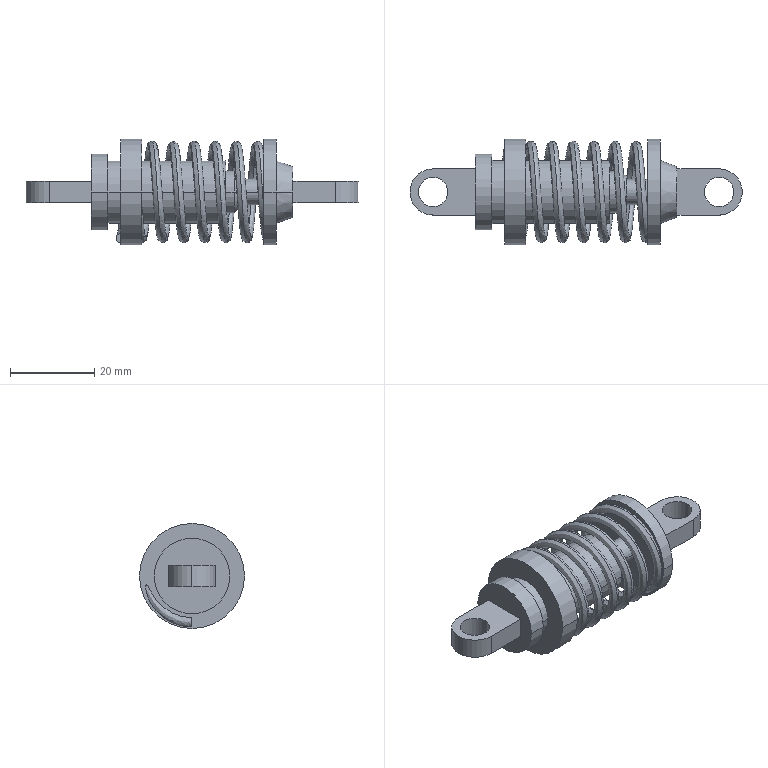Part | SolidWorks | features Extrusion 1, Helix 1, Revolution 1, Sweep 1 | 1 solid | 56 faces | box 79 x 25 x 25 mm | volume 12692 mm3 | plane 26 | cylinder 23 | cone 4 | spline 3 | commonest cylinder face diameters 7 x4 15 x4 25 x4 11 x3 6 x2 8 x2